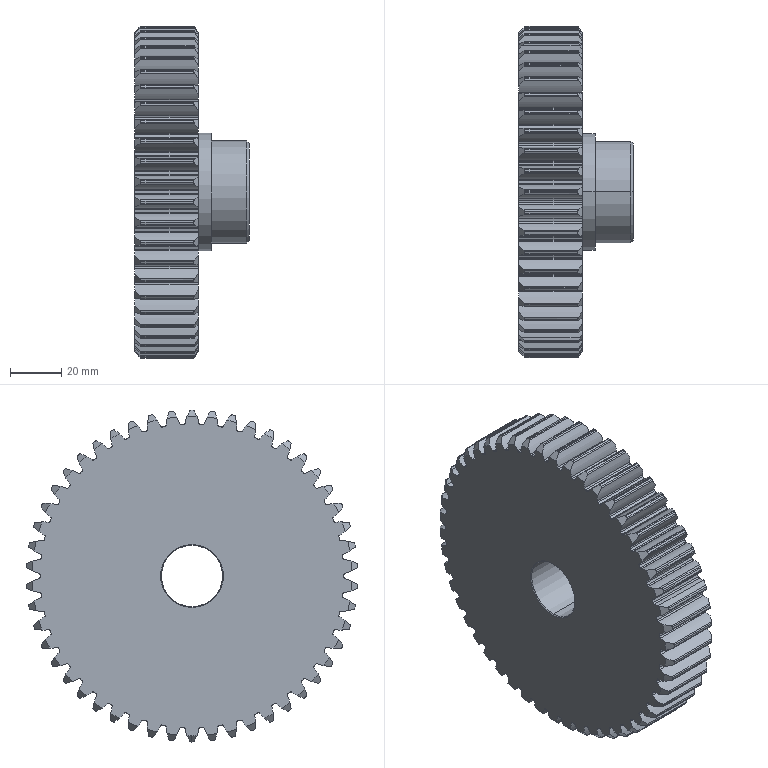Part | SolidWorks | features ICE 5, Chamfer 2, CirPattern 1, Extrusion 1, Fillet 1, RevCut 1 | 3 solids | 569 faces | box 45 x 129.796 x 130 mm | volume 311137 mm3 | cylinder 455 | cone 108 | plane 6 | commonest cylinder face diameters 1.25 x238 32.381 x106 130 x51 119 x50 24 x4 40 x4